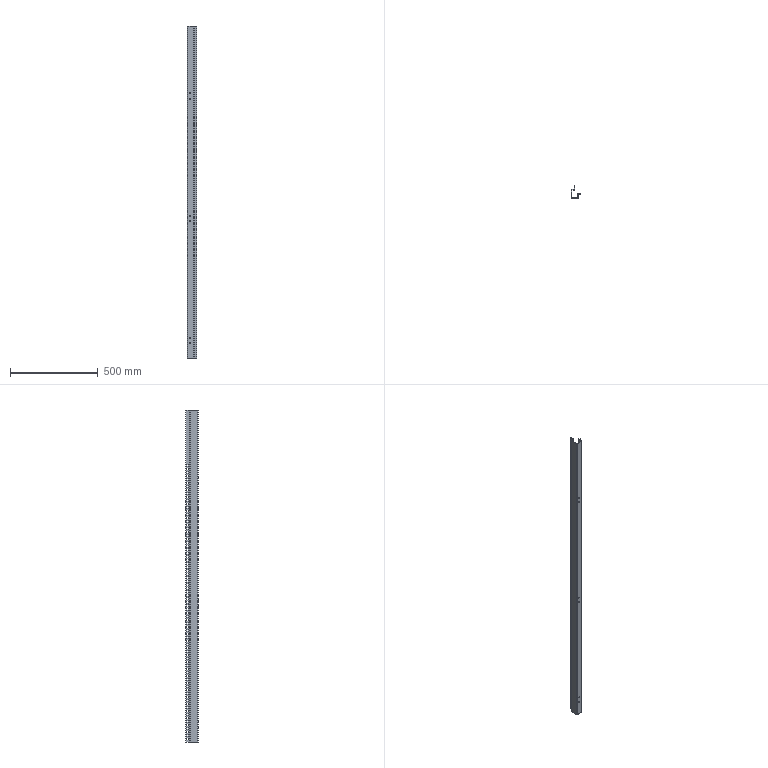Part | SolidWorks | features ICE 2, FlatPattern 1, SMBaseFlange 1, SheetMetal 1 | 1 solid | 374 faces | box 54 x 73 x 1895 mm | volume 607316 mm3 | plane 352 | cylinder 22 | commonest cylinder face diameters 6 x17 2 x5